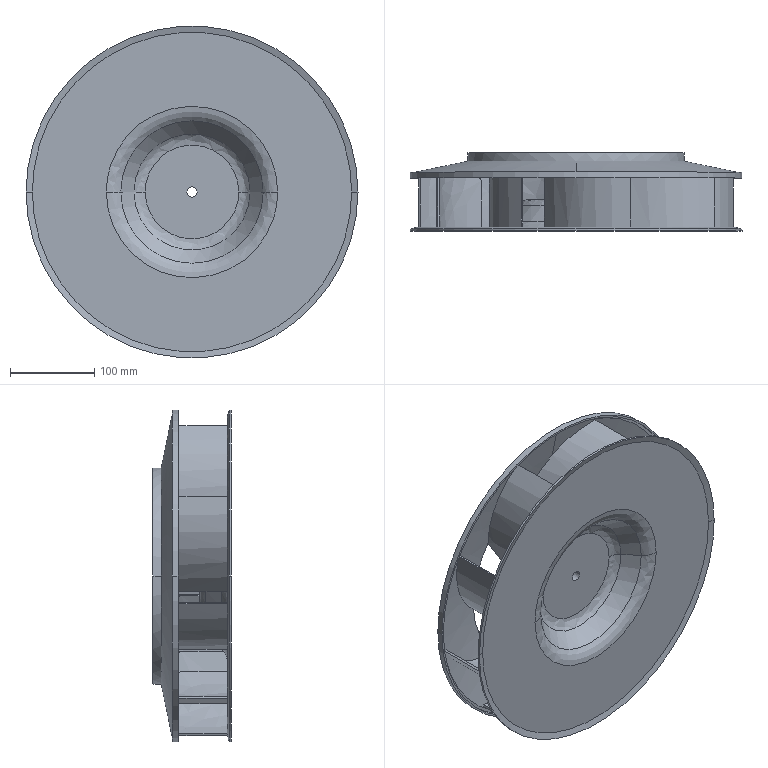Part | SolidWorks | features BaseBody 1 | 1 solid | 93 faces | box 395 x 93 x 395 mm | volume 708479 mm3 | plane 28 | spline 26 | cone 23 | cylinder 16 | commonest cylinder face diameters 395 x4 12 x2 33 x2 38 x2 253.4 x2 258 x2